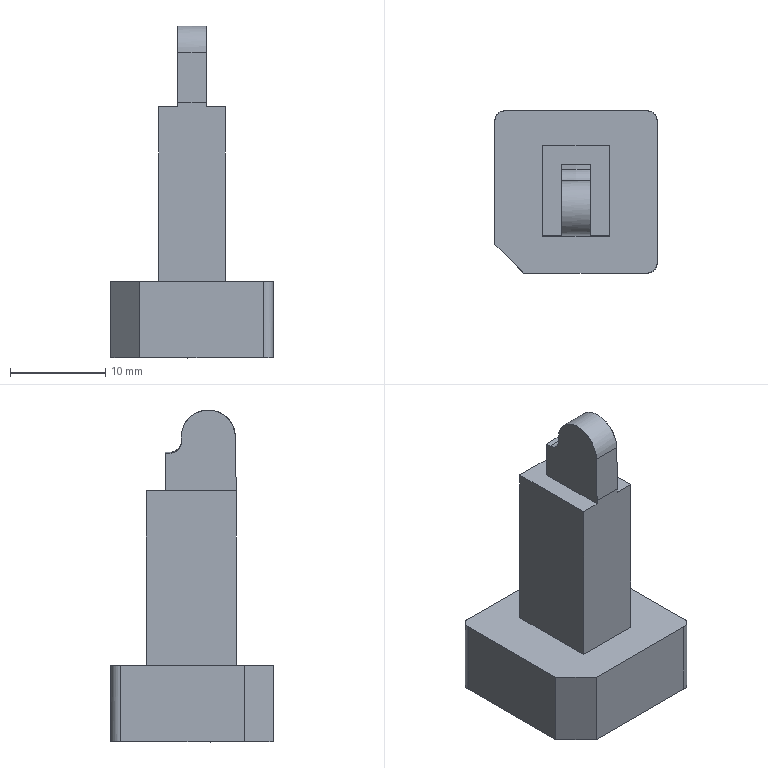NC program | PowerMill | posted with a generic post | part box 17 x 17 x 34.811 mm
Lines 6407 to 7329 of 55221:
N6504 M6
N6505 S8500 M03
N6506 G00 G90 X0.0 Y0.0
N6507 G43 Z11.798 H3
N6508
N6509 G05 P10000 R8
N6510 X4.4614 Y15.4318
N6511 Z-7.5381
N6512 G01 Z-8.7381 F360.0
N6513 X3.9497 Y10.1817 F600.0
N6514 X4.1227 Y7.5173
N6515 X3.8896 Y7.64
N6516 X3.6118 Y7.7674
N6517 X3.3339 Y7.8767
N6518 X3.1033 Y7.954
N6519 X2.7783 Y8.0439
N6520 X2.5005 Y8.1038
N6521 X2.2226 Y8.1486
N6522 X1.9448 Y8.1785
N6523 X1.667 Y8.1942
N6524 X-0.342 Y8.1963
N6525 X-0.4722 Y10.2013
N6526 X-3.4776
N6527 G03 X-4.1679 Y10.1604 I-0.0004 J-5.8404
N6528 G01 X-4.4296 Y10.1216
N6529 X-4.7432 Y10.0574
N6530 X-5.0774 Y9.9666
N6531 X-5.2425 Y9.9127
N6532 X-5.0448 Y6.8689
N6533 G00 Z4.8978
N6534 G01 X-1.8428 Y-15.2907 F10000.0
N6535 G00 Z-7.5381
N6536 G01 Z-8.7381 F360.0
N6537 Y-10.0157 F600.0
N6538 X-1.8996 Y-10.0009
N6539 X-2.2226 Y-9.9629
N6540 X-2.5005 Y-9.9183
N6541 X-2.7783 Y-9.8585
N6542 X-3.0561 Y-9.7828
N6543 X-3.3339 Y-9.691
N6544 X-3.6118 Y-9.5818
N6545 X-3.8923 Y-9.453
N6546 X-4.1688 Y-9.3061
N6547 X-4.4453 Y-9.1374
N6548 X-4.6185 Y-9.0197
N6549 X-4.7917 Y-8.8915
N6550 X-5.0009 Y-8.7217
N6551 X-5.2071 Y-8.5362
N6552 X-5.4133 Y-8.3299
N6553 X-5.5566 Y-8.1726
N6554 X-5.725 Y-7.9705
N6555 X-5.8661 Y-7.7829
N6556 X-6.0001 Y-7.5902
N6557 X-6.1185 Y-7.4007
N6558 X-6.23 Y-7.2069
N6559 X-6.3729 Y-6.9262
N6560 X-6.4953 Y-6.6454
N6561 X-6.5885 Y-6.3975
N6562 X-6.6869 Y-6.0839
N6563 X-6.7576 Y-5.8031
N6564 X-6.8125 Y-5.5224
N6565 X-6.852 Y-5.2416
N6566 X-6.8768 Y-4.9609
N6567 X-6.8868 Y-4.3993
N6568 X-6.8863 Y2.9003
N6569 X-6.8746 Y3.1811
N6570 X-6.848 Y3.4619
N6571 X-6.8064 Y3.7426
N6572 X-6.7498 Y4.0234
N6573 X-6.6679 Y4.3354
N6574 X-6.5878 Y4.5849
N6575 X-6.4812 Y4.8656
N6576 X-6.3561 Y5.1464
N6577 X-6.2413 Y5.3719
N6578 X-6.1122 Y5.5974
N6579 X-6.0436 Y5.7079
N6580 X-5.8519 Y5.9887
N6581 X-5.6114 Y6.2949
N6582 X-5.3369 Y6.5945
N6583 X-5.0883 Y6.8309
N6584 X-5.0009 Y6.9072
N6585 X-4.7231 Y7.1292
N6586 X-4.4453 Y7.3231
N6587 X-4.3359 Y7.3925
N6588 X-4.1128 Y7.5231
N6589 X-3.8896 Y7.64
N6590 X-3.6118 Y7.7674
N6591 X-3.3339 Y7.8767
N6592 X-3.1033 Y7.954
N6593 X-2.7783 Y8.0439
N6594 X-2.5005 Y8.1038
N6595 X-2.2226 Y8.1486
N6596 X-1.9448 Y8.1785
N6597 X-1.667 Y8.1942
N6598 X1.667
N6599 X1.9448 Y8.1785
N6600 X2.2226 Y8.1486
N6601 X2.5005 Y8.1038
N6602 X2.7783 Y8.0439
N6603 X3.1033 Y7.954
N6604 X3.3339 Y7.8767
N6605 X3.6118 Y7.7674
N6606 X3.8896 Y7.64
N6607 X4.1128 Y7.5231
N6608 X4.3359 Y7.3925
N6609 X4.4453 Y7.3231
N6610 X4.7231 Y7.1292
N6611 X5.0009 Y6.9072
N6612 X5.0883 Y6.8309
N6613 X5.337 Y6.5945
N6614 X5.5566 Y6.358
N6615 X5.6325 Y6.2694
N6616 X5.852 Y5.9887
N6617 X6.0436 Y5.7079
N6618 X6.1122 Y5.5974
N6619 X6.2413 Y5.3719
N6620 X6.3561 Y5.1464
N6621 X6.4814 Y4.8656
N6622 X6.5878 Y4.5849
N6623 X6.6679 Y4.3354
N6624 X6.7498 Y4.0234
N6625 X6.8064 Y3.7426
N6626 X6.848 Y3.4619
N6627 X6.8744 Y3.1811
N6628 X6.8863 Y2.9003
N6629 X6.8868 Y-4.6801
N6630 X6.8768 Y-4.9609
N6631 X6.8522 Y-5.2416
N6632 X6.8125 Y-5.5224
N6633 X6.7577 Y-5.8031
N6634 X6.6679 Y-6.1497
N6635 X6.5884 Y-6.3975
N6636 X6.4953 Y-6.6454
N6637 X6.3727 Y-6.9262
N6638 X6.23 Y-7.2069
N6639 X6.1122 Y-7.412
N6640 X5.9998 Y-7.5902
N6641 X5.8773 Y-7.7684
N6642 X5.7249 Y-7.9705
N6643 X5.5566 Y-8.1726
N6644 X5.4133 Y-8.3299
N6645 X5.2071 Y-8.5362
N6646 X5.0009 Y-8.7217
N6647 X4.7917 Y-8.8915
N6648 X4.6185 Y-9.0197
N6649 X4.4453 Y-9.1374
N6650 X4.1688 Y-9.3061
N6651 X3.8896 Y-9.4543
N6652 X3.6118 Y-9.5818
N6653 X3.3339 Y-9.691
N6654 X3.0561 Y-9.7828
N6655 X2.7783 Y-9.8585
N6656 X2.5005 Y-9.9183
N6657 X2.2226 Y-9.9629
N6658 X1.9448 Y-9.9931
N6659 X1.713 Y-10.0077
N6660 X1.667 Y-10.0157
N6661 G00 Z11.798
N6662 G05 P0
N6663 (---------------)
N6664 ( END TOOLPATH : 精公基准台01-平坦面平行-D10 )
N6665 (---------------)
N6666 ( START TOOLPATH : 精公基准台01-基准面偏置-D10 )
N6667 (---------------)
N6668 G00 X0.0 Y0.0 Z9.801
N6669 G05 P10000 R8
N6670 X-18.5956 Y11.0811
N6671 Z-25.81
N6672 G01 Z-27.01 F360.0
N6673 X-13.5737 Y9.4667 F600.0
N6674 X-8.8867 Y0.0928
N6675 Y4.8163
N6676 X-8.8794 Y5.0978
N6677 X-8.8573 Y5.3786
N6678 X-8.8205 Y5.6579
N6679 X-8.7692 Y5.9348
N6680 X-8.7034 Y6.2087
N6681 X-8.6234 Y6.4788
N6682 X-8.5294 Y6.7443
N6683 X-8.4216 Y7.0045
N6684 X-8.3004 Y7.2587
N6685 X-8.166 Y7.5063
N6686 X-8.0188 Y7.7464
N6687 X-7.8593 Y7.9786
N6688 X-7.6878 Y8.202
N6689 X-7.5049 Y8.4162
N6690 X-7.311 Y8.6205
N6691 X-7.1067 Y8.8144
N6692 X-6.8925 Y8.9973
N6693 X-6.669 Y9.1688
N6694 X-6.4369 Y9.3283
N6695 X-6.1967 Y9.4755
N6696 X-5.9492 Y9.6099
N6697 X-5.695 Y9.7311
N6698 X-5.4348 Y9.8389
N6699 X-5.1693 Y9.933
N6700 X-4.8992 Y10.013
N6701 X-4.6253 Y10.0787
N6702 X-4.3484 Y10.13
N6703 X-4.0691 Y10.1668
N6704 X-3.7883 Y10.1889
N6705 X-3.5067 Y10.1963
N6706 X3.5068
N6707 X3.7883 Y10.1889
N6708 X4.0691 Y10.1668
N6709 X4.3484 Y10.13
N6710 X4.6253 Y10.0787
N6711 X4.8992 Y10.013
N6712 G02 X5.4348 Y9.8389 I-1.6241 J-5.9094
N6713 G01 X5.695 Y9.7312
N6714 X5.9492 Y9.6099
N6715 G02 X6.669 Y9.1688 I-2.6338 J-5.1059
N6716 G01 X6.8925 Y8.9973
N6717 X7.1067 Y8.8144
N6718 X7.311 Y8.6205
N6719 X7.5049 Y8.4162
N6720 X7.6878 Y8.202
N6721 X7.8593 Y7.9786
N6722 X8.0188 Y7.7464
N6723 X8.166 Y7.5063
N6724 X8.3004 Y7.2588
N6725 X8.4216 Y7.0045
N6726 X8.5294 Y6.7443
N6727 X8.6234 Y6.4788
N6728 X8.7034 Y6.2087
N6729 G02 X8.8205 Y5.6579 I-6.2299 J-1.6122
N6730 G01 X8.8573 Y5.3786
N6731 X8.8794 Y5.0979
N6732 X8.8867 Y4.8163
N6733 Y-4.6307
N6734 X8.8794 Y-4.9123
N6735 X8.8573 Y-5.1931
N6736 X8.8205 Y-5.4723
N6737 X8.7692 Y-5.7493
N6738 X8.7034 Y-6.0232
N6739 X8.6234 Y-6.2932
N6740 X8.5294 Y-6.5588
N6741 X8.4216 Y-6.819
N6742 X8.3004 Y-7.0732
N6743 X8.166 Y-7.3207
N6744 X8.0188 Y-7.5609
N6745 X7.8593 Y-7.793
N6746 X7.6878 Y-8.0165
N6747 X7.5049 Y-8.2307
N6748 X7.311 Y-8.435
N6749 X7.1067 Y-8.6288
N6750 X6.8925 Y-8.8118
N6751 X6.669 Y-8.9832
N6752 X6.4369 Y-9.1428
N6753 X6.1967 Y-9.2899
N6754 X5.9492 Y-9.4243
N6755 X5.695 Y-9.5456
N6756 X5.4348 Y-9.6534
N6757 X5.1693 Y-9.7474
N6758 X4.8992 Y-9.8274
N6759 X4.6253 Y-9.8932
N6760 X4.2913 Y-9.952
N6761 X4.0691 Y-9.9812
N6762 G02 X3.5067 Y-10.0107 I-0.6154 J6.3606
N6763 G01 X-3.5068
N6764 X-3.7883 Y-10.0034
N6765 X-4.0691 Y-9.9813
N6766 X-4.3484 Y-9.9445
N6767 X-4.6253 Y-9.8932
N6768 X-4.8992 Y-9.8274
N6769 X-5.1693 Y-9.7474
N6770 G02 X-5.695 Y-9.5456 I2.0443 J6.111
N6771 G01 X-5.9492 Y-9.4243
N6772 G02 X-6.669 Y-8.9832 I2.624 J5.0899
N6773 G01 X-6.8925 Y-8.8118
N6774 X-7.1067 Y-8.6289
N6775 X-7.311 Y-8.435
N6776 X-7.5049 Y-8.2306
N6777 X-7.6878 Y-8.0165
N6778 X-7.8593 Y-7.793
N6779 X-8.0188 Y-7.5609
N6780 X-8.166 Y-7.3207
N6781 X-8.3004 Y-7.0732
N6782 X-8.4216 Y-6.819
N6783 X-8.5294 Y-6.5587
N6784 X-8.6234 Y-6.2932
N6785 X-8.7032 Y-6.0242
N6786 X-8.7692 Y-5.7493
N6787 X-8.8205 Y-5.4724
N6788 X-8.8573 Y-5.1931
N6789 X-8.8794 Y-4.9123
N6790 X-8.8868 Y-4.6307
N6791 X-8.8867 Y0.0928
N6792 G00 Z9.801
N6793 G05 P0
N6794 (---------------)
N6795 ( END TOOLPATH : 精公基准台01-基准面偏置-D10 )
N6796 (---------------)
N6797 ( START TOOLPATH : 精公基准台01-外形侧光-D10 )
N6798 (---------------)
N6799 G00 X0.0 Y0.0 Z10.798
N6800 G05 P10000 R8
N6801 X8.2324 Y-7.5437
N6802 Z-11.891
N6803 G01 Z-13.091 F360.0
N6804 G03 X7.1904 Y-8.0259 I0.061 J-1.4988 F600.0
N6805 G02 X3.4686 Y-9.6407 I-3.6851 J3.3969
N6806 G01 X-3.4695
N6807 G02 X-8.5167 Y-4.5639 I-0.0358 J5.0117
N6808 G01 Y4.747
N6809 G02 X-3.4686 Y9.8263 I5.0114 J0.0675
N6810 G01 X0.0003
N6811 X3.4695
N6812 G02 X8.5167 Y4.7465 I0.0358 J-5.0118
N6813 G01 Y0.0913
N6814 Y-4.5645
N6815 G02 X7.1904 Y-8.0259 I-5.0114 J-0.0645
N6816 G03 X6.7946 Y-9.1035 I1.103 J-1.0166
N6817 G01 X8.178 Y-7.4823
N6818 G03 X7.1368 Y-7.966 I0.0633 J-1.4986
N6819 G02 X3.4686 Y-9.5607 I-3.6314 J3.3369
N6820 G01 X-3.4686
N6821 G02 X-8.4367 Y-4.5639 I-0.0368 J4.9317
N6822 G01 Y4.7465
N6823 G02 X-3.4686 Y9.7463 I4.9314 J0.068
N6824 G01 X0.0003
N6825 X3.4686
N6826 G02 X8.4367 Y4.7465 I0.0367 J-4.9318
N6827 G01 Y0.0913
N6828 Y-4.5639
N6829 G02 X7.1368 Y-7.966 I-4.9313 J-0.0652
N6830 G03 X6.7427 Y-9.0443 I1.1045 J-1.0149
N6831 G00 Z10.798
N6832 X8.2324 Y-7.5437
N6833 Z1.998
N6834 G01 Z-26.98 F360.0
N6835 G03 X7.1905 Y-8.0259 I0.061 J-1.4988 F600.0
N6836 G02 X3.4686 Y-9.6407 I-3.6852 J3.3969
N6837 G01 X1.8837
N6838 X-3.4695
N6839 G02 X-8.5168 Y-4.5639 I-0.0358 J5.0117
N6840 G01 Y4.747
N6841 G02 X-3.4686 Y9.8263 I5.0115 J0.0675
N6842 G01 X3.4695
N6843 G02 X8.5168 Y4.7465 I0.0358 J-5.0118
N6844 G01 X8.5167 Y-4.5645
N6845 G02 X7.1905 Y-8.0259 I-5.0114 J-0.0645
N6846 G03 X6.7946 Y-9.1035 I1.1029 J-1.0166
N6847 G01 X8.178 Y-7.4823
N6848 G03 X7.1368 Y-7.966 I0.0633 J-1.4987
N6849 G02 X3.4686 Y-9.5607 I-3.6314 J3.337
N6850 G01 X1.8837
N6851 X-3.4686
N6852 G02 X-8.4368 Y-4.5639 I-0.0368 J4.9317
N6853 G01 Y4.7465
N6854 G02 X-3.4686 Y9.7463 I4.9315 J0.068
N6855 G01 X3.4686
N6856 G02 X8.4368 Y4.7465 I0.0367 J-4.9318
N6857 G01 Y-4.5639
N6858 G02 X7.1368 Y-7.966 I-4.9314 J-0.0651
N6859 G03 X6.7427 Y-9.0443 I1.1045 J-1.015
N6860 G00 Z10.798
N6861 G05 P0
N6862 (---------------)
N6863 ( END TOOLPATH : 精公基准台01-外形侧光-D10 )
N6864 (---------------)
N6865 ( START TOOLPATH : 精公基准台01-基准台侧光-D10 )
N6866 (---------------)
N6867 G00 X0.0 Y0.0 Z9.801
N6868 G05 P10000 R8
N6869 X13.8225 Y-16.5952
N6870 Z-33.71
N6871 G01 Z-34.91 F360.0
N6872 G03 X10.9846 Y-12.4786 I-1.419 J2.0583 F600.0
N6873 G01 X10.7944 Y-12.6097
N6874 X10.7928 Y-12.6108
N6875 X10.7913 Y-12.6118
N6876 X10.6278 Y-12.7137
N6877 X10.6266 Y-12.7144
N6878 X10.6255 Y-12.715
N6879 X10.4729 Y-12.8035
N6880 X10.4714 Y-12.8043
N6881 X10.4698 Y-12.8052
N6882 X10.1537 Y-12.9703
N6883 X10.1516 Y-12.9713
N6884 X10.1495 Y-12.9723
N6885 X9.8333 Y-13.1144
N6886 X9.8312 Y-13.1153
N6887 X9.8291 Y-13.1162
N6888 X9.5129 Y-13.237
N6889 X9.5107 Y-13.2379
N6890 X9.5084 Y-13.2386
N6891 X9.1403 Y-13.3544
N6892 X9.1383 Y-13.3551
N6893 X9.1361 Y-13.3556
N6894 X8.8719 Y-13.4232
N6895 X8.8699 Y-13.4237
N6896 X8.8678 Y-13.4241
N6897 X8.5517 Y-13.4876
N6898 X8.5497 Y-13.488
N6899 X8.5478 Y-13.4883
N6900 X8.2317 Y-13.5357
N6901 X8.2294 Y-13.536
N6902 X8.2271 Y-13.5363
N6903 X7.911 Y-13.5653
N6904 X7.909 Y-13.5655
N6905 X7.9071 Y-13.5656
N6906 X7.5909 Y-13.5792
N6907 X7.5892
N6908 X7.5875
N6909 X-5.3745 Y-13.58
N6910 X-5.3749
N6911 X-5.3754
N6912 X-5.6915 Y-13.5764
N6913 X-5.6939 Y-13.5763
N6914 X-5.6962 Y-13.5762
N6915 X-6.0124 Y-13.5541
N6916 X-6.0149 Y-13.5538
N6917 X-6.0174 Y-13.5535
N6918 X-6.3336 Y-13.5111
N6919 X-6.3361 Y-13.5107
N6920 X-6.3386 Y-13.5103
N6921 X-6.6548 Y-13.447
N6922 X-6.6573 Y-13.4464
N6923 X-6.6598 Y-13.4458
N6924 X-6.976 Y-13.3608
N6925 X-6.9785 Y-13.3601
N6926 X-6.981 Y-13.3593
N6927 X-7.2972 Y-13.2514
N6928 X-7.2997 Y-13.2505
N6929 X-7.3022 Y-13.2495
N6930 X-7.6184 Y-13.1172
N6931 X-7.6203 Y-13.1163
N6932 X-7.6223 Y-13.1154
N6933 X-7.791 Y-13.034
N6934 X-7.7923 Y-13.0334
N6935 X-7.7936 Y-13.0328
N6936 X-7.9409 Y-12.9551
N6937 X-7.9428 Y-12.9541
N6938 X-7.9447 Y-12.953
N6939 X-8.2608 Y-12.7643
N6940 X-8.2624 Y-12.7633
N6941 X-8.2639 Y-12.7623
N6942 X-8.3391 Y-12.7126
N6943 X-8.3404 Y-12.7117
N6944 X-8.3417 Y-12.7108
N6945 X-8.5826 Y-12.5378
N6946 X-8.5843 Y-12.5365
N6947 X-8.5859 Y-12.5352
N6948 X-8.7646 Y-12.3921
N6949 X-8.7659 Y-12.3911
N6950 X-8.7671 Y-12.39
N6951 X-8.9046 Y-12.2703
N6952 X-8.906 Y-12.269
N6953 X-8.9074 Y-12.2678
N6954 X-9.1128 Y-12.0714
N6955 X-9.1135 Y-12.0707
N6956 X-9.1141 Y-12.0701
N6957 X-12.0701 Y-9.1141
N6958 X-12.0707 Y-9.1135
N6959 X-12.0714 Y-9.1128
N6960 X-12.2678 Y-8.9074
N6961 X-12.269 Y-8.906
N6962 X-12.2703 Y-8.9046
N6963 X-12.39 Y-8.7671
N6964 X-12.3911 Y-8.7659
N6965 X-12.3921 Y-8.7646
N6966 X-12.5352 Y-8.5859
N6967 X-12.5365 Y-8.5843
N6968 X-12.5378 Y-8.5826
N6969 X-12.7108 Y-8.3417
N6970 X-12.7117 Y-8.3404
N6971 X-12.7126 Y-8.3391
N6972 X-12.7623 Y-8.2639
N6973 X-12.7633 Y-8.2624
N6974 X-12.7643 Y-8.2608
N6975 X-12.953 Y-7.9447
N6976 X-12.9541 Y-7.9428
N6977 X-12.9551 Y-7.9409
N6978 X-13.0328 Y-7.7936
N6979 X-13.0334 Y-7.7923
N6980 X-13.034 Y-7.791
N6981 X-13.1154 Y-7.6223
N6982 X-13.1163 Y-7.6203
N6983 X-13.1172 Y-7.6184
N6984 X-13.2495 Y-7.3022
N6985 X-13.2505 Y-7.2998
N6986 X-13.2514 Y-7.2973
N6987 X-13.3538 Y-6.9989
N6988 X-13.3546 Y-6.9964
N6989 X-13.3553 Y-6.9939
N6990 X-13.4457 Y-6.66
N6991 X-13.4464 Y-6.6574
N6992 X-13.447 Y-6.6548
N6993 X-13.5103 Y-6.3386
N6994 X-13.5107 Y-6.3361
N6995 X-13.5111 Y-6.3336
N6996 X-13.5535 Y-6.0174
N6997 X-13.5538 Y-6.0149
N6998 X-13.5541 Y-6.0124
N6999 X-13.5762 Y-5.6962
N7000 X-13.5763 Y-5.6939
N7001 X-13.5764 Y-5.6915
N7002 X-13.58 Y-5.3754
N7003 Y-5.3749
N7004 Y-5.3745
N7005 X-13.5792 Y7.5875
N7006 Y7.5891
N7007 Y7.5907
N7008 X-13.5663 Y7.9069
N7009 X-13.5662 Y7.909
N7010 X-13.5661 Y7.9111
N7011 X-13.5363 Y8.2273
N7012 X-13.536 Y8.2294
N7013 X-13.5357 Y8.2315
N7014 X-13.489 Y8.5476
N7015 X-13.4887 Y8.5498
N7016 X-13.4883 Y8.5519
N7017 X-13.424 Y8.868
N7018 X-13.4236 Y8.87
N7019 X-13.4232 Y8.8719
N7020 X-13.3556 Y9.1361
N7021 X-13.3551 Y9.1383
N7022 X-13.3544 Y9.1404
N7023 X-13.2385 Y9.5084
N7024 X-13.2377 Y9.5107
N7025 X-13.2369 Y9.5129
N7026 X-13.1162 Y9.8291
N7027 X-13.1155 Y9.8308
N7028 X-13.1148 Y9.8324
N7029 X-13.0353 Y10.0152
N7030 X-13.0349 Y10.0162
N7031 X-13.0344 Y10.0173
N7032 X-12.9716 Y10.1507
N7033 X-12.9708 Y10.1522
N7034 X-12.9701 Y10.1537
N7035 X-12.8052 Y10.4698
N7036 X-12.8044 Y10.4714
N7037 X-12.8035 Y10.4729
N7038 X-12.715 Y10.6255
N7039 X-12.7144 Y10.6266
N7040 X-12.7137 Y10.6277
N7041 X-12.612 Y10.7912
N7042 X-12.611 Y10.7928
N7043 X-12.6099 Y10.7943
N7044 X-12.3956 Y11.1054
N7045 X-12.394 Y11.1076
N7046 X-12.3924 Y11.1097
N7047 X-12.1383 Y11.4309
N7048 X-12.1372 Y11.4322
N7049 X-12.1362 Y11.4335
N7050 X-12.0741 Y11.5055
N7051 X-12.0732 Y11.5065
N7052 X-12.0722 Y11.5076
N7053 X-11.846 Y11.7518
N7054 X-11.845 Y11.7529
N7055 X-11.8439 Y11.754
N7056 X-11.754 Y11.8439
N7057 X-11.7529 Y11.845
N7058 X-11.7517 Y11.846
N7059 X-11.5074 Y12.0722
N7060 X-11.5062 Y12.0733
N7061 X-11.505 Y12.0744
N7062 X-11.4332 Y12.1357
N7063 X-11.4321 Y12.1367
N7064 X-11.431 Y12.1376
N7065 X-11.1148 Y12.3886
N7066 X-11.1127 Y12.3902
N7067 X-11.1105 Y12.3918
N7068 X-10.7944 Y12.6097
N7069 X-10.7928 Y12.6108
N7070 X-10.7913 Y12.6118
N7071 X-10.6278 Y12.7137
N7072 X-10.6266 Y12.7144
N7073 X-10.6255 Y12.715
N7074 X-10.4729 Y12.8035
N7075 X-10.4714 Y12.8043
N7076 X-10.4698 Y12.8052
N7077 X-10.1537 Y12.9703
N7078 X-10.1516 Y12.9713
N7079 X-10.1495 Y12.9723
N7080 X-9.8333 Y13.1144
N7081 X-9.8312 Y13.1153
N7082 X-9.8291 Y13.1162
N7083 X-9.5129 Y13.237
N7084 X-9.5108 Y13.2378
N7085 X-9.5087 Y13.2385
N7086 X-9.1926 Y13.3396
N7087 X-9.1905 Y13.3402
N7088 X-9.1884 Y13.3408
N7089 X-8.8722 Y13.4231
N7090 X-8.87 Y13.4236
N7091 X-8.8678 Y13.4241
N7092 X-8.5517 Y13.4876
N7093 X-8.5497 Y13.488
N7094 X-8.5478 Y13.4883
N7095 X-8.2317 Y13.5357
N7096 X-8.2294 Y13.536
N7097 X-8.2271 Y13.5363
N7098 X-7.911 Y13.5653
N7099 X-7.909 Y13.5655
N7100 X-7.9071 Y13.5656
N7101 X-7.5909 Y13.5792
N7102 X-7.5892
N7103 X-7.5875
N7104 X7.5875
N7105 X7.5891
N7106 X7.5907
N7107 X7.9069 Y13.5663
N7108 X7.909 Y13.5662
N7109 X7.9111 Y13.5661
N7110 X8.2273 Y13.5363
N7111 X8.2294 Y13.536
N7112 X8.2315 Y13.5357
N7113 X8.5476 Y13.489
N7114 X8.5498 Y13.4887
N7115 X8.5519 Y13.4883
N7116 X8.868 Y13.424
N7117 X8.87 Y13.4236
N7118 X8.8719 Y13.4232
N7119 X9.1361 Y13.3556
N7120 X9.1383 Y13.3551
N7121 X9.1404 Y13.3544
N7122 X9.5084 Y13.2385
N7123 X9.5107 Y13.2377
N7124 X9.5129 Y13.2369
N7125 X9.8291 Y13.1162
N7126 X9.8308 Y13.1155
N7127 X9.8324 Y13.1148
N7128 X10.0152 Y13.0353
N7129 X10.0162 Y13.0349
N7130 X10.0173 Y13.0344
N7131 X10.1507 Y12.9716
N7132 X10.1522 Y12.9708
N7133 X10.1537 Y12.9701
N7134 X10.4698 Y12.8052
N7135 X10.4714 Y12.8044
N7136 X10.4729 Y12.8035
N7137 X10.6255 Y12.715
N7138 X10.6266 Y12.7144
N7139 X10.6277 Y12.7137
N7140 X10.7912 Y12.612
N7141 X10.7928 Y12.611
N7142 X10.7943 Y12.6099
N7143 X11.1054 Y12.3956
N7144 X11.1076 Y12.394
N7145 X11.1097 Y12.3924
N7146 X11.4309 Y12.1383
N7147 X11.4322 Y12.1372
N7148 X11.4335 Y12.1362
N7149 X11.5055 Y12.0741
N7150 X11.5065 Y12.0732
N7151 X11.5076 Y12.0722
N7152 X11.7518 Y11.846
N7153 X11.7529 Y11.845
N7154 X11.754 Y11.8439
N7155 X11.8439 Y11.754
N7156 X11.845 Y11.7529
N7157 X11.846 Y11.7517
N7158 X12.0722 Y11.5074
N7159 X12.0733 Y11.5062
N7160 X12.0744 Y11.505
N7161 X12.1357 Y11.4332
N7162 X12.1367 Y11.4321
N7163 X12.1376 Y11.431
N7164 X12.3886 Y11.1148
N7165 X12.3902 Y11.1127
N7166 X12.3918 Y11.1105
N7167 X12.6097 Y10.7944
N7168 X12.6108 Y10.7928
N7169 X12.6118 Y10.7913
N7170 X12.7137 Y10.6278
N7171 X12.7144 Y10.6266
N7172 X12.715 Y10.6255
N7173 X12.8035 Y10.4729
N7174 X12.8043 Y10.4714
N7175 X12.8052 Y10.4698
N7176 X12.9703 Y10.1537
N7177 X12.9713 Y10.1516
N7178 X12.9723 Y10.1495
N7179 X13.1144 Y9.8333
N7180 X13.1153 Y9.8312
N7181 X13.1162 Y9.8291
N7182 X13.237 Y9.5129
N7183 X13.2378 Y9.5108
N7184 X13.2385 Y9.5087
N7185 X13.3396 Y9.1926
N7186 X13.3402 Y9.1905
N7187 X13.3408 Y9.1884
N7188 X13.4231 Y8.8722
N7189 X13.4236 Y8.87
N7190 X13.4241 Y8.8678
N7191 X13.4876 Y8.5517
N7192 X13.488 Y8.5497
N7193 X13.4883 Y8.5478
N7194 X13.5357 Y8.2317
N7195 X13.536 Y8.2294
N7196 X13.5363 Y8.2271
N7197 X13.5653 Y7.911
N7198 X13.5655 Y7.909
N7199 X13.5656 Y7.9071
N7200 X13.5792 Y7.5909
N7201 Y7.5892
N7202 Y7.5875
N7203 Y0.0
N7204 Y-7.5875
N7205 Y-7.5891
N7206 Y-7.5907
N7207 X13.5663 Y-7.9069
N7208 X13.5662 Y-7.909
N7209 X13.5661 Y-7.9112
N7210 X13.5363 Y-8.2273
N7211 X13.536 Y-8.2294
N7212 X13.5357 Y-8.2315
N7213 X13.489 Y-8.5476
N7214 X13.4887 Y-8.5498
N7215 X13.4883 Y-8.5519
N7216 X13.424 Y-8.868
N7217 X13.4236 Y-8.87
N7218 X13.4231 Y-8.8719
N7219 X13.3556 Y-9.1361
N7220 X13.3551 Y-9.1383
N7221 X13.3544 Y-9.1404
N7222 X13.2385 Y-9.5084
N7223 X13.2377 Y-9.5107
N7224 X13.2369 Y-9.5129
N7225 X13.1162 Y-9.8291
N7226 X13.1155 Y-9.8307
N7227 X13.1148 Y-9.8324
N7228 X13.0353 Y-10.0152
N7229 X13.0349 Y-10.0162
N7230 X13.0344 Y-10.0173
N7231 X12.9716 Y-10.1507
N7232 X12.9708 Y-10.1522
N7233 X12.9701 Y-10.1537
N7234 X12.8052 Y-10.4698
N7235 X12.8044 Y-10.4714
N7236 X12.8035 Y-10.4729
N7237 X12.715 Y-10.6255
N7238 X12.7144 Y-10.6266
N7239 X12.7137 Y-10.6277
N7240 X12.612 Y-10.7912
N7241 X12.611 Y-10.7928
N7242 X12.6099 Y-10.7943
N7243 X12.3956 Y-11.1054
N7244 X12.394 Y-11.1076
N7245 X12.3924 Y-11.1097
N7246 X12.1383 Y-11.4309
N7247 X12.1372 Y-11.4322
N7248 X12.1362 Y-11.4335
N7249 X12.0741 Y-11.5055
N7250 X12.0732 Y-11.5065
N7251 X12.0722 Y-11.5076
N7252 X11.846 Y-11.7518
N7253 X11.845 Y-11.7529
N7254 X11.8439 Y-11.754
N7255 X11.754 Y-11.8439
N7256 X11.7529 Y-11.845
N7257 X11.7517 Y-11.846
N7258 X11.5074 Y-12.0722
N7259 X11.5062 Y-12.0733
N7260 X11.505 Y-12.0744
N7261 X11.4332 Y-12.1357
N7262 X11.4321 Y-12.1367
N7263 X11.431 Y-12.1376
N7264 X11.1148 Y-12.3886
N7265 X11.1127 Y-12.3902
N7266 X11.1105 Y-12.3918
N7267 X10.9846 Y-12.4786
N7268 G03 X13.8225 Y-16.5952 I1.4189 J-2.0583
N7269 G01 X13.7711 Y-16.5335
N7270 G03 X10.9332 Y-12.4169 I-1.419 J2.0583
N7271 G01 X10.749 Y-12.5439
N7272 X10.5854 Y-12.6458
N7273 X10.4328 Y-12.7343
N7274 X10.1167 Y-12.8994
N7275 X9.8005 Y-13.0415
N7276 X9.4844 Y-13.1623
N7277 X9.1163 Y-13.2781
N7278 X8.8521 Y-13.3457
N7279 X8.5359 Y-13.4092
N7280 X8.2198 Y-13.4566
N7281 X7.9036 Y-13.4857
N7282 X7.5875 Y-13.4992
N7283 X7.2714 Y-13.5
N7284 X-5.3745
N7285 X-5.6906 Y-13.4964
N7286 X-6.0068 Y-13.4743
N7287 X-6.3229 Y-13.4318
N7288 X-6.6391 Y-13.3685
N7289 X-6.9552 Y-13.2836
N7290 X-7.2714 Y-13.1757
N7291 X-7.5875 Y-13.0434
N7292 X-7.7563 Y-12.962
N7293 X-7.9036 Y-12.8844
N7294 X-8.2198 Y-12.6956
N7295 X-8.295 Y-12.6458
N7296 X-8.5359 Y-12.4728
N7297 X-8.7146 Y-12.3297
N7298 X-8.8521 Y-12.2099
N7299 X-9.0575 Y-12.0135
N7300 X-12.0135 Y-9.0575
N7301 X-12.2099 Y-8.8521
N7302 X-12.3297 Y-8.7146
N7303 X-12.4728 Y-8.5359
N7304 X-12.6458 Y-8.295
N7305 X-12.6956 Y-8.2198
N7306 X-12.8844 Y-7.9036
N7307 X-12.962 Y-7.7563
N7308 X-13.0434 Y-7.5875
N7309 X-13.1757 Y-7.2714
N7310 X-13.2781 Y-6.973
N7311 X-13.3685 Y-6.6391
N7312 X-13.4318 Y-6.3229
N7313 X-13.4743 Y-6.0068
N7314 X-13.4964 Y-5.6906
N7315 X-13.5 Y-5.3745
N7316 Y7.2714
N7317 X-13.4992 Y7.5875
N7318 X-13.4864 Y7.9036
N7319 X-13.4566 Y8.2198
N7320 X-13.4099 Y8.5359
N7321 X-13.3456 Y8.8521
N7322 X-13.2781 Y9.1163
N7323 X-13.1622 Y9.4844
N7324 X-13.0415 Y9.8005
N7325 X-12.962 Y9.9832
N7326 X-12.8992 Y10.1167
N7327 X-12.7343 Y10.4328
N7328 X-12.6458 Y10.5854
N7329 X-12.544 Y10.749
N7330 X-12.3297 Y11.06
N7331 X-12.0756 Y11.3812
N7332 X-12.0135 Y11.4532
N7333 X-11.7873 Y11.6974
N7334 X-11.6974 Y11.7873
N7335 X-11.4531 Y12.0135
N7336 X-11.3812 Y12.0749
N7337 X-11.0651 Y12.3259
N7338 X-10.749 Y12.5439
N7339 X-10.5854 Y12.6458
N7340 X-10.4328 Y12.7343
N7341 X-10.1167 Y12.8994
N7342 X-9.8005 Y13.0415
N7343 X-9.4844 Y13.1623
N7344 X-9.1682 Y13.2634
N7345 X-8.8521 Y13.3457
N7346 X-8.5359 Y13.4092
N7347 X-8.2198 Y13.4566
N7348 X-7.9036 Y13.4857
N7349 X-7.5875 Y13.4992
N7350 X-7.2714 Y13.5
N7351 X7.2714
N7352 X7.5875 Y13.4992
N7353 X7.9036 Y13.4864
N7354 X8.2198 Y13.4566
N7355 X8.5359 Y13.4099
N7356 X8.8521 Y13.3456
N7357 X9.1163 Y13.2781
N7358 X9.4844 Y13.1622
N7359 X9.8005 Y13.0415
N7360 X9.9832 Y12.962
N7361 X10.1167 Y12.8992
N7362 X10.4328 Y12.7343
N7363 X10.5854 Y12.6458
N7364 X10.749 Y12.544
N7365 X11.06 Y12.3297
N7366 X11.3812 Y12.0756
N7367 X11.4532 Y12.0135
N7368 X11.6974 Y11.7873
N7369 X11.7873 Y11.6974
N7370 X12.0135 Y11.4531
N7371 X12.0749 Y11.3812
N7372 X12.3259 Y11.0651
N7373 X12.5439 Y10.749
N7374 X12.6458 Y10.5854
N7375 X12.7343 Y10.4328
N7376 X12.8994 Y10.1167
N7377 X13.0415 Y9.8005
N7378 X13.1623 Y9.4844
N7379 X13.2634 Y9.1682
N7380 X13.3457 Y8.8521
N7381 X13.4092 Y8.5359
N7382 X13.4566 Y8.2198
N7383 X13.4857 Y7.9036
N7384 X13.4992 Y7.5875
N7385 X13.5 Y7.2714
N7386 Y0.0
N7387 Y-7.2714
N7388 X13.4992 Y-7.5875
N7389 X13.4864 Y-7.9036
N7390 X13.4566 Y-8.2198
N7391 X13.4099 Y-8.5359
N7392 X13.3456 Y-8.8521
N7393 X13.2781 Y-9.1163
N7394 X13.1622 Y-9.4844
N7395 X13.0415 Y-9.8005
N7396 X12.962 Y-9.9832
N7397 X12.8992 Y-10.1167
N7398 X12.7343 Y-10.4328
N7399 X12.6458 Y-10.5854
N7400 X12.544 Y-10.749
N7401 X12.3297 Y-11.06
N7402 X12.0756 Y-11.3812
N7403 X12.0135 Y-11.4532
N7404 X11.7873 Y-11.6974
N7405 X11.6974 Y-11.7873
N7406 X11.4531 Y-12.0135
N7407 X11.3812 Y-12.0749
N7408 X11.0651 Y-12.3259
N7409 X10.9332 Y-12.4169
N7410 G03 X13.7711 Y-16.5335 I1.4189 J-2.0583
N7411 G00 Z9.801
N7412 G05 P0
N7413 (---------------)
N7414 ( END TOOLPATH : 精公基准台01-基准台侧光-D10 )
N7415 (---------------)
N7416
N7417 M05
N7418 G53 Z0.0
N7419 (---------------)
N7420 ( START TOOLPATH : 精公精光01-平行-R1 )
N7421 (---------------)
N7422 ( TOOL NO.    :4 )
N7423 ( TOOL TYPE   : BALLNOSED)
N7424 ( TOOL ID     : R1_1_1)
N7425 ( TOOL DIA    : 2.0 LENGTH 59.84)
N7426 T4